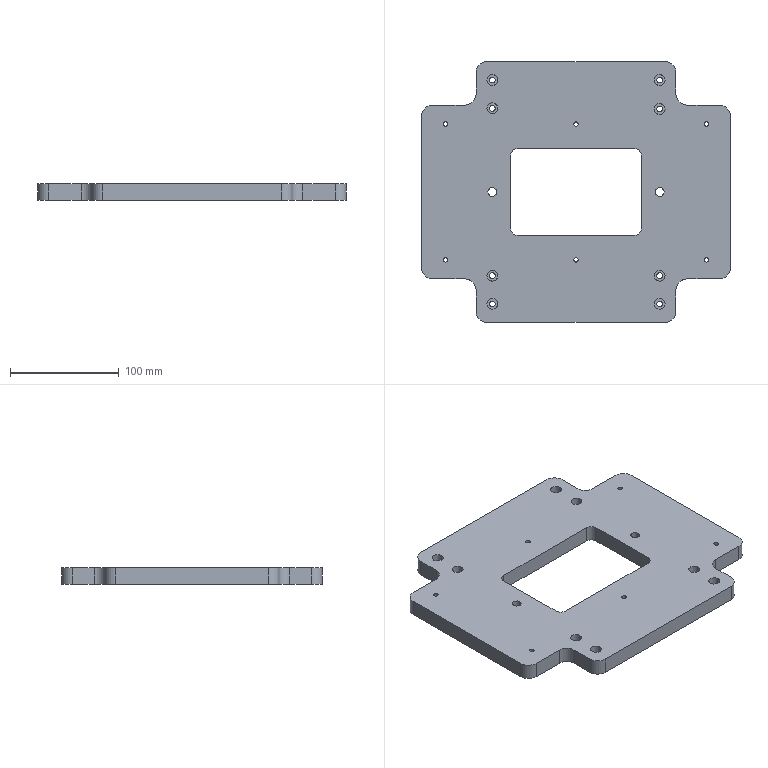NC program | NX | posted with a generic post | part box 284 x 240 x 15 mm
Lines 1 to 2692 of 2949, first 2174 of 2672 lines:
N10 G17 G21 G94 G90
(DRILLING , TOOL : D6A45)
N12 T07 M6
N14 G54
N16 G17 G0 G90 X0. Y-62.5 S5000 M3
N18 G43 Z30. H7
N20 G94 G81 G98 Z-1. F250. R3.
N22 X-77. Y-103.
N24 Y-77.
N26 X-120. Y-62.5
N28 X-77. Y0.
N30 X-120. Y62.5
N32 X-77. Y77.
N34 Y103.
N36 X0. Y62.5
N38 X77. Y103.
N40 Y76.337
N42 X120. Y62.5
N44 X77. Y0.
N46 X120. Y-62.5
N48 X77. Y-77.
N50 Y-103.
N52 G80
N54 G0 X77. Y-103. Z30.
N56 M5
(DRILLING_COPY , TOOL : 4.2ZT)
N58 T12 M6
N60 G54
N62 G17 G0 G90 X-120. Y62.5 S2000 M3
N64 G43 Z30. H12
N66 G94 G83 G98 Z-17.202 F200. Q2. R3.
N68 X0.
N70 X120.
N72 Y-62.5
N74 X0.
N76 X-120.
N78 G80
N80 G0 X-120. Y-62.5 Z30.
N82 M5
(DRILLING_COPY_1 , TOOL : 5.3ZT)
N84 T13 M6
N86 G54
N88 G17 G0 G90 X-77. Y-77. S2000 M3
N90 G43 Z30. H13
N92 G94 G83 G98 Z-17.592 F200. Q2. R3.
N94 Y-103.
N96 X77.
N98 Y-77.
N100 Y76.337
N102 Y103.
N104 X-77.
N106 Y77.
N108 G80
N110 G0 X-77. Y77. Z30.
N112 M5
(DRILLING_COPY_COPY , TOOL : 7.8ZT)
N114 T14 M6
N116 G54
N118 G17 G0 G90 X-77. Y0. S2000 M3
N120 G43 Z30. H14
N122 G94 G83 G98 Z-18.343 F200. Q2. R3.
N124 X77.
N126 G80
N128 G0 X77. Y0. Z30.
N130 M5
(HOLE_MILLING_1 , TOOL : D6)
N132 T06 M6
N134 G54
N136 G17 G0 G90 X-77. Y103. S9500 M3
N138 G43 Z30. H6
N140 Z0.5
N142 G94 G3 X-76. Y102. R1. F1600.
N144 X-75. Y103. R1.
N146 X-75. Y103. Z0. I-2. J0.
N148 X-75. Y103. Z-0.5 I-2. J0.
N150 X-75. Y103. Z-1. I-2. J0.
N152 X-75. Y103. Z-1.5 I-2. J0.
N154 X-75. Y103. Z-2. I-2. J0.
N156 X-75. Y103. Z-2.5 I-2. J0.
N158 X-75. Y103. Z-3. I-2. J0.
N160 X-75. Y103. Z-3.5 I-2. J0.
N162 X-75. Y103. Z-4. I-2. J0.
N164 X-75. Y103. Z-4.5 I-2. J0.
N166 X-75. Y103. Z-5. I-2. J0.
N168 X-75. Y103. Z-5.5 I-2. J0.
N170 X-75. Y103. Z-6. I-2. J0.
N172 X-75. Y103. Z-6.5 I-2. J0.
N174 X-75. Y103. Z-7. I-2. J0.
N176 X-75. Y103. Z-7.5 I-2. J0.
N178 X-75. Y103. Z-8. I-2. J0.
N180 X-75. Y103. Z-8.5 I-2. J0.
N182 X-75. Y103. Z-9. I-2. J0.
N184 X-75. Y103. Z-9.5 I-2. J0.
N186 X-75. Y103. Z-10. I-2. J0.
N188 X-75. Y103. Z-10.5 I-2. J0.
N190 X-75. Y103. Z-11. I-2. J0.
N192 X-75. Y103. Z-11.5 I-2. J0.
N194 X-75. Y103. Z-12. I-2. J0.
N196 X-77. Y105. R2.
N198 X-75. Y103. R-2.
N200 X-76. Y104. R1.
N202 X-77. Y103. R1.
N204 G0 Z30.
N206 Y77.
N208 Z0.5
N210 G3 X-76. Y76. R1.
N212 X-75. Y77. R1.
N214 X-75. Y77. Z0. I-2. J0.
N216 X-75. Y77. Z-0.5 I-2. J0.
N218 X-75. Y77. Z-1. I-2. J0.
N220 X-75. Y77. Z-1.5 I-2. J0.
N222 X-75. Y77. Z-2. I-2. J0.
N224 X-75. Y77. Z-2.5 I-2. J0.
N226 X-75. Y77. Z-3. I-2. J0.
N228 X-75. Y77. Z-3.5 I-2. J0.
N230 X-75. Y77. Z-4. I-2. J0.
N232 X-75. Y77. Z-4.5 I-2. J0.
N234 X-75. Y77. Z-5. I-2. J0.
N236 X-75. Y77. Z-5.5 I-2. J0.
N238 X-75. Y77. Z-6. I-2. J0.
N240 X-75. Y77. Z-6.5 I-2. J0.
N242 X-75. Y77. Z-7. I-2. J0.
N244 X-75. Y77. Z-7.5 I-2. J0.
N246 X-75. Y77. Z-8. I-2. J0.
N248 X-75. Y77. Z-8.5 I-2. J0.
N250 X-75. Y77. Z-9. I-2. J0.
N252 X-75. Y77. Z-9.5 I-2. J0.
N254 X-75. Y77. Z-10. I-2. J0.
N256 X-75. Y77. Z-10.5 I-2. J0.
N258 X-75. Y77. Z-11. I-2. J0.
N260 X-75. Y77. Z-11.5 I-2. J0.
N262 X-75. Y77. Z-12. I-2. J0.
N264 X-77. Y79. R2.
N266 X-75. Y77. R-2.
N268 X-76. Y78. R1.
N270 X-77. Y77. R1.
N272 G0 Z30.
N274 Y-77.
N276 Z0.5
N278 G3 X-76. Y-78. R1.
N280 X-75. Y-77. R1.
N282 X-75. Y-77. Z0. I-2. J0.
N284 X-75. Y-77. Z-0.5 I-2. J0.
N286 X-75. Y-77. Z-1. I-2. J0.
N288 X-75. Y-77. Z-1.5 I-2. J0.
N290 X-75. Y-77. Z-2. I-2. J0.
N292 X-75. Y-77. Z-2.5 I-2. J0.
N294 X-75. Y-77. Z-3. I-2. J0.
N296 X-75. Y-77. Z-3.5 I-2. J0.
N298 X-75. Y-77. Z-4. I-2. J0.
N300 X-75. Y-77. Z-4.5 I-2. J0.
N302 X-75. Y-77. Z-5. I-2. J0.
N304 X-75. Y-77. Z-5.5 I-2. J0.
N306 X-75. Y-77. Z-6. I-2. J0.
N308 X-75. Y-77. Z-6.5 I-2. J0.
N310 X-75. Y-77. Z-7. I-2. J0.
N312 X-75. Y-77. Z-7.5 I-2. J0.
N314 X-75. Y-77. Z-8. I-2. J0.
N316 X-75. Y-77. Z-8.5 I-2. J0.
N318 X-75. Y-77. Z-9. I-2. J0.
N320 X-75. Y-77. Z-9.5 I-2. J0.
N322 X-75. Y-77. Z-10. I-2. J0.
N324 X-75. Y-77. Z-10.5 I-2. J0.
N326 X-75. Y-77. Z-11. I-2. J0.
N328 X-75. Y-77. Z-11.5 I-2. J0.
N330 X-75. Y-77. Z-12. I-2. J0.
N332 X-77. Y-75. R2.
N334 X-75. Y-77. R-2.
N336 X-76. Y-76. R1.
N338 X-77. Y-77. R1.
N340 G0 Z30.
N342 Y-103.
N344 Z0.5
N346 G3 X-76. Y-104. R1.
N348 X-75. Y-103. R1.
N350 X-75. Y-103. Z0. I-2. J0.
N352 X-75. Y-103. Z-0.5 I-2. J0.
N354 X-75. Y-103. Z-1. I-2. J0.
N356 X-75. Y-103. Z-1.5 I-2. J0.
N358 X-75. Y-103. Z-2. I-2. J0.
N360 X-75. Y-103. Z-2.5 I-2. J0.
N362 X-75. Y-103. Z-3. I-2. J0.
N364 X-75. Y-103. Z-3.5 I-2. J0.
N366 X-75. Y-103. Z-4. I-2. J0.
N368 X-75. Y-103. Z-4.5 I-2. J0.
N370 X-75. Y-103. Z-5. I-2. J0.
N372 X-75. Y-103. Z-5.5 I-2. J0.
N374 X-75. Y-103. Z-6. I-2. J0.
N376 X-75. Y-103. Z-6.5 I-2. J0.
N378 X-75. Y-103. Z-7. I-2. J0.
N380 X-75. Y-103. Z-7.5 I-2. J0.
N382 X-75. Y-103. Z-8. I-2. J0.
N384 X-75. Y-103. Z-8.5 I-2. J0.
N386 X-75. Y-103. Z-9. I-2. J0.
N388 X-75. Y-103. Z-9.5 I-2. J0.
N390 X-75. Y-103. Z-10. I-2. J0.
N392 X-75. Y-103. Z-10.5 I-2. J0.
N394 X-75. Y-103. Z-11. I-2. J0.
N396 X-75. Y-103. Z-11.5 I-2. J0.
N398 X-75. Y-103. Z-12. I-2. J0.
N400 X-77. Y-101. R2.
N402 X-75. Y-103. R-2.
N404 X-76. Y-102. R1.
N406 X-77. Y-103. R1.
N408 G0 Z30.
N410 X77.
N412 Z0.5
N414 G3 X78. Y-104. R1.
N416 X79. Y-103. R1.
N418 X79. Y-103. Z0. I-2. J0.
N420 X79. Y-103. Z-0.5 I-2. J0.
N422 X79. Y-103. Z-1. I-2. J0.
N424 X79. Y-103. Z-1.5 I-2. J0.
N426 X79. Y-103. Z-2. I-2. J0.
N428 X79. Y-103. Z-2.5 I-2. J0.
N430 X79. Y-103. Z-3. I-2. J0.
N432 X79. Y-103. Z-3.5 I-2. J0.
N434 X79. Y-103. Z-4. I-2. J0.
N436 X79. Y-103. Z-4.5 I-2. J0.
N438 X79. Y-103. Z-5. I-2. J0.
N440 X79. Y-103. Z-5.5 I-2. J0.
N442 X79. Y-103. Z-6. I-2. J0.
N444 X79. Y-103. Z-6.5 I-2. J0.
N446 X79. Y-103. Z-7. I-2. J0.
N448 X79. Y-103. Z-7.5 I-2. J0.
N450 X79. Y-103. Z-8. I-2. J0.
N452 X79. Y-103. Z-8.5 I-2. J0.
N454 X79. Y-103. Z-9. I-2. J0.
N456 X79. Y-103. Z-9.5 I-2. J0.
N458 X79. Y-103. Z-10. I-2. J0.
N460 X79. Y-103. Z-10.5 I-2. J0.
N462 X79. Y-103. Z-11. I-2. J0.
N464 X79. Y-103. Z-11.5 I-2. J0.
N466 X79. Y-103. Z-12. I-2. J0.
N468 X77. Y-101. R2.
N470 X79. Y-103. R-2.
N472 X78. Y-102. R1.
N474 X77. Y-103. R1.
N476 G0 Z30.
N478 Y-77.
N480 Z0.5
N482 G3 X78. Y-78. R1.
N484 X79. Y-77. R1.
N486 X79. Y-77. Z0. I-2. J0.
N488 X79. Y-77. Z-0.5 I-2. J0.
N490 X79. Y-77. Z-1. I-2. J0.
N492 X79. Y-77. Z-1.5 I-2. J0.
N494 X79. Y-77. Z-2. I-2. J0.
N496 X79. Y-77. Z-2.5 I-2. J0.
N498 X79. Y-77. Z-3. I-2. J0.
N500 X79. Y-77. Z-3.5 I-2. J0.
N502 X79. Y-77. Z-4. I-2. J0.
N504 X79. Y-77. Z-4.5 I-2. J0.
N506 X79. Y-77. Z-5. I-2. J0.
N508 X79. Y-77. Z-5.5 I-2. J0.
N510 X79. Y-77. Z-6. I-2. J0.
N512 X79. Y-77. Z-6.5 I-2. J0.
N514 X79. Y-77. Z-7. I-2. J0.
N516 X79. Y-77. Z-7.5 I-2. J0.
N518 X79. Y-77. Z-8. I-2. J0.
N520 X79. Y-77. Z-8.5 I-2. J0.
N522 X79. Y-77. Z-9. I-2. J0.
N524 X79. Y-77. Z-9.5 I-2. J0.
N526 X79. Y-77. Z-10. I-2. J0.
N528 X79. Y-77. Z-10.5 I-2. J0.
N530 X79. Y-77. Z-11. I-2. J0.
N532 X79. Y-77. Z-11.5 I-2. J0.
N534 X79. Y-77. Z-12. I-2. J0.
N536 X77. Y-75. R2.
N538 X79. Y-77. R-2.
N540 X78. Y-76. R1.
N542 X77. Y-77. R1.
N544 G0 Z30.
N546 Y76.337
N548 Z0.5
N550 G3 X78. Y75.337 R1.
N552 X79. Y76.337 R1.
N554 X79. Y76.337 Z0. I-2. J0.
N556 X79. Y76.337 Z-0.5 I-2. J0.
N558 X79. Y76.337 Z-1. I-2. J0.
N560 X79. Y76.337 Z-1.5 I-2. J0.
N562 X79. Y76.337 Z-2. I-2. J0.
N564 X79. Y76.337 Z-2.5 I-2. J0.
N566 X79. Y76.337 Z-3. I-2. J0.
N568 X79. Y76.337 Z-3.5 I-2. J0.
N570 X79. Y76.337 Z-4. I-2. J0.
N572 X79. Y76.337 Z-4.5 I-2. J0.
N574 X79. Y76.337 Z-5. I-2. J0.
N576 X79. Y76.337 Z-5.5 I-2. J0.
N578 X79. Y76.337 Z-6. I-2. J0.
N580 X79. Y76.337 Z-6.5 I-2. J0.
N582 X79. Y76.337 Z-7. I-2. J0.
N584 X79. Y76.337 Z-7.5 I-2. J0.
N586 X79. Y76.337 Z-8. I-2. J0.
N588 X79. Y76.337 Z-8.5 I-2. J0.
N590 X79. Y76.337 Z-9. I-2. J0.
N592 X79. Y76.337 Z-9.5 I-2. J0.
N594 X79. Y76.337 Z-10. I-2. J0.
N596 X79. Y76.337 Z-10.5 I-2. J0.
N598 X79. Y76.337 Z-11. I-2. J0.
N600 X79. Y76.337 Z-11.5 I-2. J0.
N602 X79. Y76.337 Z-12. I-2. J0.
N604 X77. Y78.337 R2.
N606 X79. Y76.337 R-2.
N608 X78. Y77.337 R1.
N610 X77. Y76.337 R1.
N612 G0 Z30.
N614 Y103.
N616 Z0.5
N618 G3 X78. Y102. R1.
N620 X79. Y103. R1.
N622 X79. Y103. Z0. I-2. J0.
N624 X79. Y103. Z-0.5 I-2. J0.
N626 X79. Y103. Z-1. I-2. J0.
N628 X79. Y103. Z-1.5 I-2. J0.
N630 X79. Y103. Z-2. I-2. J0.
N632 X79. Y103. Z-2.5 I-2. J0.
N634 X79. Y103. Z-3. I-2. J0.
N636 X79. Y103. Z-3.5 I-2. J0.
N638 X79. Y103. Z-4. I-2. J0.
N640 X79. Y103. Z-4.5 I-2. J0.
N642 X79. Y103. Z-5. I-2. J0.
N644 X79. Y103. Z-5.5 I-2. J0.
N646 X79. Y103. Z-6. I-2. J0.
N648 X79. Y103. Z-6.5 I-2. J0.
N650 X79. Y103. Z-7. I-2. J0.
N652 X79. Y103. Z-7.5 I-2. J0.
N654 X79. Y103. Z-8. I-2. J0.
N656 X79. Y103. Z-8.5 I-2. J0.
N658 X79. Y103. Z-9. I-2. J0.
N660 X79. Y103. Z-9.5 I-2. J0.
N662 X79. Y103. Z-10. I-2. J0.
N664 X79. Y103. Z-10.5 I-2. J0.
N666 X79. Y103. Z-11. I-2. J0.
N668 X79. Y103. Z-11.5 I-2. J0.
N670 X79. Y103. Z-12. I-2. J0.
N672 X77. Y105. R2.
N674 X79. Y103. R-2.
N676 X78. Y104. R1.
N678 X77. Y103. R1.
N680 G0 Z30.
N682 M5
(PLANAR_MILL , TOOL : D10)
N684 T10 M6
N686 G54
N688 G17 G0 G90 X3.438 Y-0.4 S9500 M3
N690 G43 Z30. H10
N692 Z1.5
N694 G94 G1 X20.4 Z0.611 F1000.
N696 Y0.4 Z0.569
N698 X0. Z-0.5
N700 X-20.4 F3000.
N702 Y-0.4
N704 X20.4
N706 Y0.4
N708 X0.
N710 Y4.9
N712 X-24.9
N714 Y-4.9
N716 X24.9
N718 Y4.9
N720 X0.
N722 Y10.9
N724 X-30.9
N726 Y-10.9
N728 X30.9
N730 Y10.9
N732 X0.
N734 Y16.9
N736 X-36.9
N738 Y-16.9
N740 X36.9
N742 Y16.9
N744 X0.
N746 Y22.9
N748 X-42.9
N750 Y-22.9
N752 X42.9
N754 Y22.9
N756 X0.
N758 Y28.9
N760 X-48.9
N762 Y-28.9
N764 X48.9
N766 Y28.9
N768 X0.
N770 Y34.9
N772 X-54.
N774 G3 X-54.9 Y34. R0.9
N776 G1 Y-34.
N778 G3 X-54. Y-34.9 R0.9
N780 G1 X54.
N782 G3 X54.9 Y-34. R0.9
N784 G1 Y34.
N786 G3 X54. Y34.9 R0.9
N788 G1 X0.
N790 Z1.
N792 G0 X3.438 Y-0.4
N794 G1 X20.4 Z0.111 F1000.
N796 Y0.4 Z0.069
N798 X0. Z-1.
N800 X-20.4 F3000.
N802 Y-0.4
N804 X20.4
N806 Y0.4
N808 X0.
N810 Y4.9
N812 X-24.9
N814 Y-4.9
N816 X24.9
N818 Y4.9
N820 X0.
N822 Y10.9
N824 X-30.9
N826 Y-10.9
N828 X30.9
N830 Y10.9
N832 X0.
N834 Y16.9
N836 X-36.9
N838 Y-16.9
N840 X36.9
N842 Y16.9
N844 X0.
N846 Y22.9
N848 X-42.9
N850 Y-22.9
N852 X42.9
N854 Y22.9
N856 X0.
N858 Y28.9
N860 X-48.9
N862 Y-28.9
N864 X48.9
N866 Y28.9
N868 X0.
N870 Y34.9
N872 X-54.
N874 G3 X-54.9 Y34. R0.9
N876 G1 Y-34.
N878 G3 X-54. Y-34.9 R0.9
N880 G1 X54.
N882 G3 X54.9 Y-34. R0.9
N884 G1 Y34.
N886 G3 X54. Y34.9 R0.9
N888 G1 X0.
N890 Z0.5
N892 G0 X3.438 Y-0.4
N894 G1 X20.4 Z-0.389 F1000.
N896 Y0.4 Z-0.431
N898 X0. Z-1.5
N900 X-20.4 F3000.
N902 Y-0.4
N904 X20.4
N906 Y0.4
N908 X0.
N910 Y4.9
N912 X-24.9
N914 Y-4.9
N916 X24.9
N918 Y4.9
N920 X0.
N922 Y10.9
N924 X-30.9
N926 Y-10.9
N928 X30.9
N930 Y10.9
N932 X0.
N934 Y16.9
N936 X-36.9
N938 Y-16.9
N940 X36.9
N942 Y16.9
N944 X0.
N946 Y22.9
N948 X-42.9
N950 Y-22.9
N952 X42.9
N954 Y22.9
N956 X0.
N958 Y28.9
N960 X-48.9
N962 Y-28.9
N964 X48.9
N966 Y28.9
N968 X0.
N970 Y34.9
N972 X-54.
N974 G3 X-54.9 Y34. R0.9
N976 G1 Y-34.
N978 G3 X-54. Y-34.9 R0.9
N980 G1 X54.
N982 G3 X54.9 Y-34. R0.9
N984 G1 Y34.
N986 G3 X54. Y34.9 R0.9
N988 G1 X0.
N990 Z0.
N992 G0 X3.438 Y-0.4
N994 G1 X20.4 Z-0.889 F1000.
N996 Y0.4 Z-0.931
N998 X0. Z-2.
N1000 X-20.4 F3000.
N1002 Y-0.4
N1004 X20.4
N1006 Y0.4
N1008 X0.
N1010 Y4.9
N1012 X-24.9
N1014 Y-4.9
N1016 X24.9
N1018 Y4.9
N1020 X0.
N1022 Y10.9
N1024 X-30.9
N1026 Y-10.9
N1028 X30.9
N1030 Y10.9
N1032 X0.
N1034 Y16.9
N1036 X-36.9
N1038 Y-16.9
N1040 X36.9
N1042 Y16.9
N1044 X0.
N1046 Y22.9
N1048 X-42.9
N1050 Y-22.9
N1052 X42.9
N1054 Y22.9
N1056 X0.
N1058 Y28.9
N1060 X-48.9
N1062 Y-28.9
N1064 X48.9
N1066 Y28.9
N1068 X0.
N1070 Y34.9
N1072 X-54.
N1074 G3 X-54.9 Y34. R0.9
N1076 G1 Y-34.
N1078 G3 X-54. Y-34.9 R0.9
N1080 G1 X54.
N1082 G3 X54.9 Y-34. R0.9
N1084 G1 Y34.
N1086 G3 X54. Y34.9 R0.9
N1088 G1 X0.
N1090 Z-0.5
N1092 G0 X3.438 Y-0.4
N1094 G1 X20.4 Z-1.389 F1000.
N1096 Y0.4 Z-1.431
N1098 X0. Z-2.5
N1100 X-20.4 F3000.
N1102 Y-0.4
N1104 X20.4
N1106 Y0.4
N1108 X0.
N1110 Y4.9
N1112 X-24.9
N1114 Y-4.9
N1116 X24.9
N1118 Y4.9
N1120 X0.
N1122 Y10.9
N1124 X-30.9
N1126 Y-10.9
N1128 X30.9
N1130 Y10.9
N1132 X0.
N1134 Y16.9
N1136 X-36.9
N1138 Y-16.9
N1140 X36.9
N1142 Y16.9
N1144 X0.
N1146 Y22.9
N1148 X-42.9
N1150 Y-22.9
N1152 X42.9
N1154 Y22.9
N1156 X0.
N1158 Y28.9
N1160 X-48.9
N1162 Y-28.9
N1164 X48.9
N1166 Y28.9
N1168 X0.
N1170 Y34.9
N1172 X-54.
N1174 G3 X-54.9 Y34. R0.9
N1176 G1 Y-34.
N1178 G3 X-54. Y-34.9 R0.9
N1180 G1 X54.
N1182 G3 X54.9 Y-34. R0.9
N1184 G1 Y34.
N1186 G3 X54. Y34.9 R0.9
N1188 G1 X0.
N1190 Z-1.
N1192 G0 X3.438 Y-0.4
N1194 G1 X20.4 Z-1.889 F1000.
N1196 Y0.4 Z-1.931
N1198 X0. Z-3.
N1200 X-20.4 F3000.
N1202 Y-0.4
N1204 X20.4
N1206 Y0.4
N1208 X0.
N1210 Y4.9
N1212 X-24.9
N1214 Y-4.9
N1216 X24.9
N1218 Y4.9
N1220 X0.
N1222 Y10.9
N1224 X-30.9
N1226 Y-10.9
N1228 X30.9
N1230 Y10.9
N1232 X0.
N1234 Y16.9
N1236 X-36.9
N1238 Y-16.9
N1240 X36.9
N1242 Y16.9
N1244 X0.
N1246 Y22.9
N1248 X-42.9
N1250 Y-22.9
N1252 X42.9
N1254 Y22.9
N1256 X0.
N1258 Y28.9
N1260 X-48.9
N1262 Y-28.9
N1264 X48.9
N1266 Y28.9
N1268 X0.
N1270 Y34.9
N1272 X-54.
N1274 G3 X-54.9 Y34. R0.9
N1276 G1 Y-34.
N1278 G3 X-54. Y-34.9 R0.9
N1280 G1 X54.
N1282 G3 X54.9 Y-34. R0.9
N1284 G1 Y34.
N1286 G3 X54. Y34.9 R0.9
N1288 G1 X0.
N1290 Z-1.5
N1292 G0 X3.438 Y-0.4
N1294 G1 X20.4 Z-2.389 F1000.
N1296 Y0.4 Z-2.431
N1298 X0. Z-3.5
N1300 X-20.4 F3000.
N1302 Y-0.4
N1304 X20.4
N1306 Y0.4
N1308 X0.
N1310 Y4.9
N1312 X-24.9
N1314 Y-4.9
N1316 X24.9
N1318 Y4.9
N1320 X0.
N1322 Y10.9
N1324 X-30.9
N1326 Y-10.9
N1328 X30.9
N1330 Y10.9
N1332 X0.
N1334 Y16.9
N1336 X-36.9
N1338 Y-16.9
N1340 X36.9
N1342 Y16.9
N1344 X0.
N1346 Y22.9
N1348 X-42.9
N1350 Y-22.9
N1352 X42.9
N1354 Y22.9
N1356 X0.
N1358 Y28.9
N1360 X-48.9
N1362 Y-28.9
N1364 X48.9
N1366 Y28.9
N1368 X0.
N1370 Y34.9
N1372 X-54.
N1374 G3 X-54.9 Y34. R0.9
N1376 G1 Y-34.
N1378 G3 X-54. Y-34.9 R0.9
N1380 G1 X54.
N1382 G3 X54.9 Y-34. R0.9
N1384 G1 Y34.
N1386 G3 X54. Y34.9 R0.9
N1388 G1 X0.
N1390 Z-2.
N1392 G0 X3.438 Y-0.4
N1394 G1 X20.4 Z-2.889 F1000.
N1396 Y0.4 Z-2.931
N1398 X0. Z-4.
N1400 X-20.4 F3000.
N1402 Y-0.4
N1404 X20.4
N1406 Y0.4
N1408 X0.
N1410 Y4.9
N1412 X-24.9
N1414 Y-4.9
N1416 X24.9
N1418 Y4.9
N1420 X0.
N1422 Y10.9
N1424 X-30.9
N1426 Y-10.9
N1428 X30.9
N1430 Y10.9
N1432 X0.
N1434 Y16.9
N1436 X-36.9
N1438 Y-16.9
N1440 X36.9
N1442 Y16.9
N1444 X0.
N1446 Y22.9
N1448 X-42.9
N1450 Y-22.9
N1452 X42.9
N1454 Y22.9
N1456 X0.
N1458 Y28.9
N1460 X-48.9
N1462 Y-28.9
N1464 X48.9
N1466 Y28.9
N1468 X0.
N1470 Y34.9
N1472 X-54.
N1474 G3 X-54.9 Y34. R0.9
N1476 G1 Y-34.
N1478 G3 X-54. Y-34.9 R0.9
N1480 G1 X54.
N1482 G3 X54.9 Y-34. R0.9
N1484 G1 Y34.
N1486 G3 X54. Y34.9 R0.9
N1488 G1 X0.
N1490 Z-2.5
N1492 G0 X3.438 Y-0.4
N1494 G1 X20.4 Z-3.389 F1000.
N1496 Y0.4 Z-3.431
N1498 X0. Z-4.5
N1500 X-20.4 F3000.
N1502 Y-0.4
N1504 X20.4
N1506 Y0.4
N1508 X0.
N1510 Y4.9
N1512 X-24.9
N1514 Y-4.9
N1516 X24.9
N1518 Y4.9
N1520 X0.
N1522 Y10.9
N1524 X-30.9
N1526 Y-10.9
N1528 X30.9
N1530 Y10.9
N1532 X0.
N1534 Y16.9
N1536 X-36.9
N1538 Y-16.9
N1540 X36.9
N1542 Y16.9
N1544 X0.
N1546 Y22.9
N1548 X-42.9
N1550 Y-22.9
N1552 X42.9
N1554 Y22.9
N1556 X0.
N1558 Y28.9
N1560 X-48.9
N1562 Y-28.9
N1564 X48.9
N1566 Y28.9
N1568 X0.
N1570 Y34.9
N1572 X-54.
N1574 G3 X-54.9 Y34. R0.9
N1576 G1 Y-34.
N1578 G3 X-54. Y-34.9 R0.9
N1580 G1 X54.
N1582 G3 X54.9 Y-34. R0.9
N1584 G1 Y34.
N1586 G3 X54. Y34.9 R0.9
N1588 G1 X0.
N1590 Z-3.
N1592 G0 X3.438 Y-0.4
N1594 G1 X20.4 Z-3.889 F1000.
N1596 Y0.4 Z-3.931
N1598 X0. Z-5.
N1600 X-20.4 F3000.
N1602 Y-0.4
N1604 X20.4
N1606 Y0.4
N1608 X0.
N1610 Y4.9
N1612 X-24.9
N1614 Y-4.9
N1616 X24.9
N1618 Y4.9
N1620 X0.
N1622 Y10.9
N1624 X-30.9
N1626 Y-10.9
N1628 X30.9
N1630 Y10.9
N1632 X0.
N1634 Y16.9
N1636 X-36.9
N1638 Y-16.9
N1640 X36.9
N1642 Y16.9
N1644 X0.
N1646 Y22.9
N1648 X-42.9
N1650 Y-22.9
N1652 X42.9
N1654 Y22.9
N1656 X0.
N1658 Y28.9
N1660 X-48.9
N1662 Y-28.9
N1664 X48.9
N1666 Y28.9
N1668 X0.
N1670 Y34.9
N1672 X-54.
N1674 G3 X-54.9 Y34. R0.9
N1676 G1 Y-34.
N1678 G3 X-54. Y-34.9 R0.9
N1680 G1 X54.
N1682 G3 X54.9 Y-34. R0.9
N1684 G1 Y34.
N1686 G3 X54. Y34.9 R0.9
N1688 G1 X0.
N1690 Z-3.5
N1692 G0 X3.438 Y-0.4
N1694 G1 X20.4 Z-4.389 F1000.
N1696 Y0.4 Z-4.431
N1698 X0. Z-5.5
N1700 X-20.4 F3000.
N1702 Y-0.4
N1704 X20.4
N1706 Y0.4
N1708 X0.
N1710 Y4.9
N1712 X-24.9
N1714 Y-4.9
N1716 X24.9
N1718 Y4.9
N1720 X0.
N1722 Y10.9
N1724 X-30.9
N1726 Y-10.9
N1728 X30.9
N1730 Y10.9
N1732 X0.
N1734 Y16.9
N1736 X-36.9
N1738 Y-16.9
N1740 X36.9
N1742 Y16.9
N1744 X0.
N1746 Y22.9
N1748 X-42.9
N1750 Y-22.9
N1752 X42.9
N1754 Y22.9
N1756 X0.
N1758 Y28.9
N1760 X-48.9
N1762 Y-28.9
N1764 X48.9
N1766 Y28.9
N1768 X0.
N1770 Y34.9
N1772 X-54.
N1774 G3 X-54.9 Y34. R0.9
N1776 G1 Y-34.
N1778 G3 X-54. Y-34.9 R0.9
N1780 G1 X54.
N1782 G3 X54.9 Y-34. R0.9
N1784 G1 Y34.
N1786 G3 X54. Y34.9 R0.9
N1788 G1 X0.
N1790 Z-4.
N1792 G0 X3.438 Y-0.4
N1794 G1 X20.4 Z-4.889 F1000.
N1796 Y0.4 Z-4.931
N1798 X0. Z-6.
N1800 X-20.4 F3000.
N1802 Y-0.4
N1804 X20.4
N1806 Y0.4
N1808 X0.
N1810 Y4.9
N1812 X-24.9
N1814 Y-4.9
N1816 X24.9
N1818 Y4.9
N1820 X0.
N1822 Y10.9
N1824 X-30.9
N1826 Y-10.9
N1828 X30.9
N1830 Y10.9
N1832 X0.
N1834 Y16.9
N1836 X-36.9
N1838 Y-16.9
N1840 X36.9
N1842 Y16.9
N1844 X0.
N1846 Y22.9
N1848 X-42.9
N1850 Y-22.9
N1852 X42.9
N1854 Y22.9
N1856 X0.
N1858 Y28.9
N1860 X-48.9
N1862 Y-28.9
N1864 X48.9
N1866 Y28.9
N1868 X0.
N1870 Y34.9
N1872 X-54.
N1874 G3 X-54.9 Y34. R0.9
N1876 G1 Y-34.
N1878 G3 X-54. Y-34.9 R0.9
N1880 G1 X54.
N1882 G3 X54.9 Y-34. R0.9
N1884 G1 Y34.
N1886 G3 X54. Y34.9 R0.9
N1888 G1 X0.
N1890 Z-4.5
N1892 G0 X3.438 Y-0.4
N1894 G1 X20.4 Z-5.389 F1000.
N1896 Y0.4 Z-5.431
N1898 X0. Z-6.5
N1900 X-20.4 F3000.
N1902 Y-0.4
N1904 X20.4
N1906 Y0.4
N1908 X0.
N1910 Y4.9
N1912 X-24.9
N1914 Y-4.9
N1916 X24.9
N1918 Y4.9
N1920 X0.
N1922 Y10.9
N1924 X-30.9
N1926 Y-10.9
N1928 X30.9
N1930 Y10.9
N1932 X0.
N1934 Y16.9
N1936 X-36.9
N1938 Y-16.9
N1940 X36.9
N1942 Y16.9
N1944 X0.
N1946 Y22.9
N1948 X-42.9
N1950 Y-22.9
N1952 X42.9
N1954 Y22.9
N1956 X0.
N1958 Y28.9
N1960 X-48.9
N1962 Y-28.9
N1964 X48.9
N1966 Y28.9
N1968 X0.
N1970 Y34.9
N1972 X-54.
N1974 G3 X-54.9 Y34. R0.9
N1976 G1 Y-34.
N1978 G3 X-54. Y-34.9 R0.9
N1980 G1 X54.
N1982 G3 X54.9 Y-34. R0.9
N1984 G1 Y34.
N1986 G3 X54. Y34.9 R0.9
N1988 G1 X0.
N1990 Z-5.
N1992 G0 X3.438 Y-0.4
N1994 G1 X20.4 Z-5.889 F1000.
N1996 Y0.4 Z-5.931
N1998 X0. Z-7.
N2000 X-20.4 F3000.
N2002 Y-0.4
N2004 X20.4
N2006 Y0.4
N2008 X0.
N2010 Y4.9
N2012 X-24.9
N2014 Y-4.9
N2016 X24.9
N2018 Y4.9
N2020 X0.
N2022 Y10.9
N2024 X-30.9
N2026 Y-10.9
N2028 X30.9
N2030 Y10.9
N2032 X0.
N2034 Y16.9
N2036 X-36.9
N2038 Y-16.9
N2040 X36.9
N2042 Y16.9
N2044 X0.
N2046 Y22.9
N2048 X-42.9
N2050 Y-22.9
N2052 X42.9
N2054 Y22.9
N2056 X0.
N2058 Y28.9
N2060 X-48.9
N2062 Y-28.9
N2064 X48.9
N2066 Y28.9
N2068 X0.
N2070 Y34.9
N2072 X-54.
N2074 G3 X-54.9 Y34. R0.9
N2076 G1 Y-34.
N2078 G3 X-54. Y-34.9 R0.9
N2080 G1 X54.
N2082 G3 X54.9 Y-34. R0.9
N2084 G1 Y34.
N2086 G3 X54. Y34.9 R0.9
N2088 G1 X0.
N2090 Z-5.5
N2092 G0 X3.438 Y-0.4
N2094 G1 X20.4 Z-6.389 F1000.
N2096 Y0.4 Z-6.431
N2098 X0. Z-7.5
N2100 X-20.4 F3000.
N2102 Y-0.4
N2104 X20.4
N2106 Y0.4
N2108 X0.
N2110 Y4.9
N2112 X-24.9
N2114 Y-4.9
N2116 X24.9
N2118 Y4.9
N2120 X0.
N2122 Y10.9
N2124 X-30.9
N2126 Y-10.9
N2128 X30.9
N2130 Y10.9
N2132 X0.
N2134 Y16.9
N2136 X-36.9
N2138 Y-16.9
N2140 X36.9
N2142 Y16.9
N2144 X0.
N2146 Y22.9
N2148 X-42.9
N2150 Y-22.9
N2152 X42.9
N2154 Y22.9
N2156 X0.
N2158 Y28.9
N2160 X-48.9
N2162 Y-28.9
N2164 X48.9
N2166 Y28.9
N2168 X0.
N2170 Y34.9
N2172 X-54.
N2174 G3 X-54.9 Y34. R0.9
N2176 G1 Y-34.
N2178 G3 X-54. Y-34.9 R0.9
N2180 G1 X54.
N2182 G3 X54.9 Y-34. R0.9
N2184 G1 Y34.
N2186 G3 X54. Y34.9 R0.9
N2188 G1 X0.
N2190 Z-6.
N2192 G0 X3.438 Y-0.4
N2194 G1 X20.4 Z-6.889 F1000.
N2196 Y0.4 Z-6.931
N2198 X0. Z-8.
N2200 X-20.4 F3000.
N2202 Y-0.4
N2204 X20.4
N2206 Y0.4
N2208 X0.
N2210 Y4.9
N2212 X-24.9
N2214 Y-4.9
N2216 X24.9
N2218 Y4.9
N2220 X0.
N2222 Y10.9
N2224 X-30.9
N2226 Y-10.9
N2228 X30.9
N2230 Y10.9
N2232 X0.
N2234 Y16.9
N2236 X-36.9
N2238 Y-16.9
N2240 X36.9
N2242 Y16.9
N2244 X0.
N2246 Y22.9
N2248 X-42.9
N2250 Y-22.9
N2252 X42.9
N2254 Y22.9
N2256 X0.
N2258 Y28.9
N2260 X-48.9
N2262 Y-28.9
N2264 X48.9
N2266 Y28.9
N2268 X0.
N2270 Y34.9
N2272 X-54.
N2274 G3 X-54.9 Y34. R0.9
N2276 G1 Y-34.
N2278 G3 X-54. Y-34.9 R0.9
N2280 G1 X54.
N2282 G3 X54.9 Y-34. R0.9
N2284 G1 Y34.
N2286 G3 X54. Y34.9 R0.9
N2288 G1 X0.
N2290 Z-6.5
N2292 G0 X3.438 Y-0.4
N2294 G1 X20.4 Z-7.389 F1000.
N2296 Y0.4 Z-7.431
N2298 X0. Z-8.5
N2300 X-20.4 F3000.
N2302 Y-0.4
N2304 X20.4
N2306 Y0.4
N2308 X0.
N2310 Y4.9
N2312 X-24.9
N2314 Y-4.9
N2316 X24.9
N2318 Y4.9
N2320 X0.
N2322 Y10.9
N2324 X-30.9
N2326 Y-10.9
N2328 X30.9
N2330 Y10.9
N2332 X0.
N2334 Y16.9
N2336 X-36.9
N2338 Y-16.9
N2340 X36.9
N2342 Y16.9
N2344 X0.
N2346 Y22.9
N2348 X-42.9
N2350 Y-22.9
N2352 X42.9
N2354 Y22.9
N2356 X0.
N2358 Y28.9
N2360 X-48.9
N2362 Y-28.9
N2364 X48.9
N2366 Y28.9
N2368 X0.
N2370 Y34.9
N2372 X-54.
N2374 G3 X-54.9 Y34. R0.9
N2376 G1 Y-34.
N2378 G3 X-54. Y-34.9 R0.9
N2380 G1 X54.
N2382 G3 X54.9 Y-34. R0.9
N2384 G1 Y34.
N2386 G3 X54. Y34.9 R0.9
N2388 G1 X0.
N2390 Z-7.
N2392 G0 X3.438 Y-0.4
N2394 G1 X20.4 Z-7.889 F1000.
N2396 Y0.4 Z-7.931
N2398 X0. Z-9.
N2400 X-20.4 F3000.
N2402 Y-0.4
N2404 X20.4
N2406 Y0.4
N2408 X0.
N2410 Y4.9
N2412 X-24.9
N2414 Y-4.9
N2416 X24.9
N2418 Y4.9
N2420 X0.
N2422 Y10.9
N2424 X-30.9
N2426 Y-10.9
N2428 X30.9
N2430 Y10.9
N2432 X0.
N2434 Y16.9
N2436 X-36.9
N2438 Y-16.9
N2440 X36.9
N2442 Y16.9
N2444 X0.
N2446 Y22.9
N2448 X-42.9
N2450 Y-22.9
N2452 X42.9
N2454 Y22.9
N2456 X0.
N2458 Y28.9
N2460 X-48.9
N2462 Y-28.9
N2464 X48.9
N2466 Y28.9
N2468 X0.
N2470 Y34.9
N2472 X-54.
N2474 G3 X-54.9 Y34. R0.9
N2476 G1 Y-34.
N2478 G3 X-54. Y-34.9 R0.9
N2480 G1 X54.
N2482 G3 X54.9 Y-34. R0.9
N2484 G1 Y34.
N2486 G3 X54. Y34.9 R0.9
N2488 G1 X0.
N2490 Z-7.5
N2492 G0 X3.438 Y-0.4
N2494 G1 X20.4 Z-8.389 F1000.
N2496 Y0.4 Z-8.431
N2498 X0. Z-9.5
N2500 X-20.4 F3000.
N2502 Y-0.4
N2504 X20.4
N2506 Y0.4
N2508 X0.
N2510 Y4.9
N2512 X-24.9
N2514 Y-4.9
N2516 X24.9
N2518 Y4.9
N2520 X0.
N2522 Y10.9
N2524 X-30.9
N2526 Y-10.9
N2528 X30.9
N2530 Y10.9
N2532 X0.
N2534 Y16.9
N2536 X-36.9
N2538 Y-16.9
N2540 X36.9
N2542 Y16.9
N2544 X0.
N2546 Y22.9
N2548 X-42.9
N2550 Y-22.9
N2552 X42.9
N2554 Y22.9
N2556 X0.
N2558 Y28.9
N2560 X-48.9
N2562 Y-28.9
N2564 X48.9
N2566 Y28.9
N2568 X0.
N2570 Y34.9
N2572 X-54.
N2574 G3 X-54.9 Y34. R0.9
N2576 G1 Y-34.
N2578 G3 X-54. Y-34.9 R0.9
N2580 G1 X54.
N2582 G3 X54.9 Y-34. R0.9
N2584 G1 Y34.
N2586 G3 X54. Y34.9 R0.9
N2588 G1 X0.
N2590 Z-8.
N2592 G0 X3.438 Y-0.4
N2594 G1 X20.4 Z-8.889 F1000.
N2596 Y0.4 Z-8.931
N2598 X0. Z-10.
N2600 X-20.4 F3000.
N2602 Y-0.4
N2604 X20.4
N2606 Y0.4
N2608 X0.
N2610 Y4.9
N2612 X-24.9
N2614 Y-4.9
N2616 X24.9
N2618 Y4.9
N2620 X0.
N2622 Y10.9
N2624 X-30.9
N2626 Y-10.9
N2628 X30.9
N2630 Y10.9
N2632 X0.
N2634 Y16.9
N2636 X-36.9
N2638 Y-16.9
N2640 X36.9
N2642 Y16.9
N2644 X0.
N2646 Y22.9
N2648 X-42.9
N2650 Y-22.9
N2652 X42.9
N2654 Y22.9
N2656 X0.
N2658 Y28.9
N2660 X-48.9
N2662 Y-28.9
N2664 X48.9
N2666 Y28.9
N2668 X0.
N2670 Y34.9
N2672 X-54.
N2674 G3 X-54.9 Y34. R0.9
N2676 G1 Y-34.
N2678 G3 X-54. Y-34.9 R0.9
N2680 G1 X54.
N2682 G3 X54.9 Y-34. R0.9
N2684 G1 Y34.
N2686 G3 X54. Y34.9 R0.9
N2688 G1 X0.
N2690 Z-8.5
N2692 G0 X3.438 Y-0.4
N2694 G1 X20.4 Z-9.389 F1000.
N2696 Y0.4 Z-9.431
N2698 X0. Z-10.5
N2700 X-20.4 F3000.
N2702 Y-0.4
N2704 X20.4
N2706 Y0.4
N2708 X0.
N2710 Y4.9
N2712 X-24.9
N2714 Y-4.9
N2716 X24.9
N2718 Y4.9
N2720 X0.
N2722 Y10.9
N2724 X-30.9
N2726 Y-10.9
N2728 X30.9
N2730 Y10.9
N2732 X0.
N2734 Y16.9
N2736 X-36.9
N2738 Y-16.9
N2740 X36.9
N2742 Y16.9
N2744 X0.
N2746 Y22.9
N2748 X-42.9
N2750 Y-22.9
N2752 X42.9
N2754 Y22.9
N2756 X0.
N2758 Y28.9
N2760 X-48.9
N2762 Y-28.9
N2764 X48.9
N2766 Y28.9
N2768 X0.
N2770 Y34.9
N2772 X-54.
N2774 G3 X-54.9 Y34. R0.9
N2776 G1 Y-34.
N2778 G3 X-54. Y-34.9 R0.9
N2780 G1 X54.
N2782 G3 X54.9 Y-34. R0.9
N2784 G1 Y34.
N2786 G3 X54. Y34.9 R0.9
N2788 G1 X0.
N2790 Z-9.
N2792 G0 X3.438 Y-0.4
N2794 G1 X20.4 Z-9.889 F1000.
N2796 Y0.4 Z-9.931
N2798 X0. Z-11.
N2800 X-20.4 F3000.
N2802 Y-0.4
N2804 X20.4
N2806 Y0.4
N2808 X0.
N2810 Y4.9
N2812 X-24.9
N2814 Y-4.9
N2816 X24.9
N2818 Y4.9
N2820 X0.
N2822 Y10.9
N2824 X-30.9
N2826 Y-10.9
N2828 X30.9
N2830 Y10.9
N2832 X0.
N2834 Y16.9
N2836 X-36.9
N2838 Y-16.9
N2840 X36.9
N2842 Y16.9
N2844 X0.
N2846 Y22.9
N2848 X-42.9
N2850 Y-22.9
N2852 X42.9
N2854 Y22.9
N2856 X0.
N2858 Y28.9
N2860 X-48.9
N2862 Y-28.9
N2864 X48.9
N2866 Y28.9
N2868 X0.
N2870 Y34.9
N2872 X-54.
N2874 G3 X-54.9 Y34. R0.9
N2876 G1 Y-34.
N2878 G3 X-54. Y-34.9 R0.9
N2880 G1 X54.
N2882 G3 X54.9 Y-34. R0.9
N2884 G1 Y34.
N2886 G3 X54. Y34.9 R0.9
N2888 G1 X0.
N2890 Z-9.5
N2892 G0 X3.438 Y-0.4
N2894 G1 X20.4 Z-10.389 F1000.
N2896 Y0.4 Z-10.431
N2898 X0. Z-11.5
N2900 X-20.4 F3000.
N2902 Y-0.4
N2904 X20.4
N2906 Y0.4
N2908 X0.
N2910 Y4.9
N2912 X-24.9
N2914 Y-4.9
N2916 X24.9
N2918 Y4.9
N2920 X0.
N2922 Y10.9
N2924 X-30.9
N2926 Y-10.9
N2928 X30.9
N2930 Y10.9
N2932 X0.
N2934 Y16.9
N2936 X-36.9
N2938 Y-16.9
N2940 X36.9
N2942 Y16.9
N2944 X0.
N2946 Y22.9
N2948 X-42.9
N2950 Y-22.9
N2952 X42.9
N2954 Y22.9
N2956 X0.
N2958 Y28.9
N2960 X-48.9
N2962 Y-28.9
N2964 X48.9
N2966 Y28.9
N2968 X0.
N2970 Y34.9
N2972 X-54.
N2974 G3 X-54.9 Y34. R0.9
N2976 G1 Y-34.
N2978 G3 X-54. Y-34.9 R0.9
N2980 G1 X54.
N2982 G3 X54.9 Y-34. R0.9
N2984 G1 Y34.
N2986 G3 X54. Y34.9 R0.9
N2988 G1 X0.
N2990 Z-10.
N2992 G0 X3.438 Y-0.4
N2994 G1 X20.4 Z-10.889 F1000.
N2996 Y0.4 Z-10.931
N2998 X0. Z-12.
N3000 X-20.4 F3000.
N3002 Y-0.4
N3004 X20.4
N3006 Y0.4
N3008 X0.
N3010 Y4.9
N3012 X-24.9
N3014 Y-4.9
N3016 X24.9
N3018 Y4.9
N3020 X0.
N3022 Y10.9
N3024 X-30.9
N3026 Y-10.9
N3028 X30.9
N3030 Y10.9
N3032 X0.
N3034 Y16.9
N3036 X-36.9
N3038 Y-16.9
N3040 X36.9
N3042 Y16.9
N3044 X0.
N3046 Y22.9
N3048 X-42.9
N3050 Y-22.9
N3052 X42.9
N3054 Y22.9
N3056 X0.
N3058 Y28.9
N3060 X-48.9
N3062 Y-28.9
N3064 X48.9
N3066 Y28.9
N3068 X0.
N3070 Y34.9
N3072 X-54.
N3074 G3 X-54.9 Y34. R0.9
N3076 G1 Y-34.
N3078 G3 X-54. Y-34.9 R0.9
N3080 G1 X54.
N3082 G3 X54.9 Y-34. R0.9
N3084 G1 Y34.
N3086 G3 X54. Y34.9 R0.9
N3088 G1 X0.
N3090 Z-10.5
N3092 G0 X3.438 Y-0.4
N3094 G1 X20.4 Z-11.389 F1000.
N3096 Y0.4 Z-11.431
N3098 X0. Z-12.5
N3100 X-20.4 F3000.
N3102 Y-0.4
N3104 X20.4
N3106 Y0.4
N3108 X0.
N3110 Y4.9
N3112 X-24.9
N3114 Y-4.9
N3116 X24.9
N3118 Y4.9
N3120 X0.
N3122 Y10.9
N3124 X-30.9
N3126 Y-10.9
N3128 X30.9
N3130 Y10.9
N3132 X0.
N3134 Y16.9
N3136 X-36.9
N3138 Y-16.9
N3140 X36.9
N3142 Y16.9
N3144 X0.
N3146 Y22.9
N3148 X-42.9
N3150 Y-22.9
N3152 X42.9
N3154 Y22.9
N3156 X0.
N3158 Y28.9
N3160 X-48.9
N3162 Y-28.9
N3164 X48.9
N3166 Y28.9
N3168 X0.
N3170 Y34.9
N3172 X-54.
N3174 G3 X-54.9 Y34. R0.9
N3176 G1 Y-34.
N3178 G3 X-54. Y-34.9 R0.9
N3180 G1 X54.
N3182 G3 X54.9 Y-34. R0.9
N3184 G1 Y34.
N3186 G3 X54. Y34.9 R0.9
N3188 G1 X0.
N3190 Z-11.
N3192 G0 X3.438 Y-0.4
N3194 G1 X20.4 Z-11.889 F1000.
N3196 Y0.4 Z-11.931
N3198 X0. Z-13.
N3200 X-20.4 F3000.
N3202 Y-0.4
N3204 X20.4
N3206 Y0.4
N3208 X0.
N3210 Y4.9
N3212 X-24.9
N3214 Y-4.9
N3216 X24.9
N3218 Y4.9
N3220 X0.
N3222 Y10.9
N3224 X-30.9
N3226 Y-10.9
N3228 X30.9
N3230 Y10.9
N3232 X0.
N3234 Y16.9
N3236 X-36.9
N3238 Y-16.9
N3240 X36.9
N3242 Y16.9
N3244 X0.
N3246 Y22.9
N3248 X-42.9
N3250 Y-22.9
N3252 X42.9
N3254 Y22.9
N3256 X0.
N3258 Y28.9
N3260 X-48.9
N3262 Y-28.9
N3264 X48.9
N3266 Y28.9
N3268 X0.
N3270 Y34.9
N3272 X-54.
N3274 G3 X-54.9 Y34. R0.9
N3276 G1 Y-34.
N3278 G3 X-54. Y-34.9 R0.9
N3280 G1 X54.
N3282 G3 X54.9 Y-34. R0.9
N3284 G1 Y34.
N3286 G3 X54. Y34.9 R0.9
N3288 G1 X0.
N3290 Z-11.5
N3292 G0 X3.438 Y-0.4
N3294 G1 X20.4 Z-12.389 F1000.
N3296 Y0.4 Z-12.431
N3298 X0. Z-13.5
N3300 X-20.4 F3000.
N3302 Y-0.4
N3304 X20.4
N3306 Y0.4
N3308 X0.
N3310 Y4.9
N3312 X-24.9
N3314 Y-4.9
N3316 X24.9
N3318 Y4.9
N3320 X0.
N3322 Y10.9
N3324 X-30.9
N3326 Y-10.9
N3328 X30.9
N3330 Y10.9
N3332 X0.
N3334 Y16.9
N3336 X-36.9
N3338 Y-16.9
N3340 X36.9
N3342 Y16.9
N3344 X0.
N3346 Y22.9
N3348 X-42.9
N3350 Y-22.9
N3352 X42.9
N3354 Y22.9
N3356 X0.
N3358 Y28.9
N3360 X-48.9
N3362 Y-28.9
N3364 X48.9
N3366 Y28.9
N3368 X0.
N3370 Y34.9
N3372 X-54.
N3374 G3 X-54.9 Y34. R0.9
N3376 G1 Y-34.
N3378 G3 X-54. Y-34.9 R0.9
N3380 G1 X54.
N3382 G3 X54.9 Y-34. R0.9
N3384 G1 Y34.
N3386 G3 X54. Y34.9 R0.9
N3388 G1 X0.
N3390 Z-12.
N3392 G0 X3.438 Y-0.4
N3394 G1 X20.4 Z-12.889 F1000.
N3396 Y0.4 Z-12.931
N3398 X0. Z-14.
N3400 X-20.4 F3000.
N3402 Y-0.4
N3404 X20.4
N3406 Y0.4
N3408 X0.
N3410 Y4.9
N3412 X-24.9
N3414 Y-4.9
N3416 X24.9
N3418 Y4.9
N3420 X0.
N3422 Y10.9
N3424 X-30.9
N3426 Y-10.9
N3428 X30.9
N3430 Y10.9
N3432 X0.
N3434 Y16.9
N3436 X-36.9
N3438 Y-16.9
N3440 X36.9
N3442 Y16.9
N3444 X0.
N3446 Y22.9
N3448 X-42.9
N3450 Y-22.9
N3452 X42.9
N3454 Y22.9
N3456 X0.
N3458 Y28.9
N3460 X-48.9
N3462 Y-28.9
N3464 X48.9
N3466 Y28.9
N3468 X0.
N3470 Y34.9
N3472 X-54.
N3474 G3 X-54.9 Y34. R0.9
N3476 G1 Y-34.
N3478 G3 X-54. Y-34.9 R0.9
N3480 G1 X54.
N3482 G3 X54.9 Y-34. R0.9
N3484 G1 Y34.
N3486 G3 X54. Y34.9 R0.9
N3488 G1 X0.
N3490 Z-12.5
N3492 G0 X3.438 Y-0.4
N3494 G1 X20.4 Z-13.389 F1000.
N3496 Y0.4 Z-13.431
N3498 X0. Z-14.5
N3500 X-20.4 F3000.
N3502 Y-0.4
N3504 X20.4
N3506 Y0.4
N3508 X0.
N3510 Y4.9
N3512 X-24.9
N3514 Y-4.9
N3516 X24.9
N3518 Y4.9
N3520 X0.
N3522 Y10.9
N3524 X-30.9
N3526 Y-10.9
N3528 X30.9
N3530 Y10.9
N3532 X0.
N3534 Y16.9
N3536 X-36.9
N3538 Y-16.9
N3540 X36.9
N3542 Y16.9
N3544 X0.
N3546 Y22.9
N3548 X-42.9
N3550 Y-22.9
N3552 X42.9
N3554 Y22.9
N3556 X0.
N3558 Y28.9
N3560 X-48.9
N3562 Y-28.9
N3564 X48.9
N3566 Y28.9
N3568 X0.
N3570 Y34.9
N3572 X-54.
N3574 G3 X-54.9 Y34. R0.9
N3576 G1 Y-34.
N3578 G3 X-54. Y-34.9 R0.9
N3580 G1 X54.
N3582 G3 X54.9 Y-34. R0.9
N3584 G1 Y34.
N3586 G3 X54. Y34.9 R0.9
N3588 G1 X0.
N3590 Z-13.
N3592 G0 X3.438 Y-0.4
N3594 G1 X20.4 Z-13.889 F1000.
N3596 Y0.4 Z-13.931
N3598 X0. Z-15.
N3600 X-20.4 F3000.
N3602 Y-0.4
N3604 X20.4
N3606 Y0.4
N3608 X0.
N3610 Y4.9
N3612 X-24.9
N3614 Y-4.9
N3616 X24.9
N3618 Y4.9
N3620 X0.
N3622 Y10.9
N3624 X-30.9
N3626 Y-10.9
N3628 X30.9
N3630 Y10.9
N3632 X0.
N3634 Y16.9
N3636 X-36.9
N3638 Y-16.9
N3640 X36.9
N3642 Y16.9
N3644 X0.
N3646 Y22.9
N3648 X-42.9
N3650 Y-22.9
N3652 X42.9
N3654 Y22.9
N3656 X0.
N3658 Y28.9
N3660 X-48.9
N3662 Y-28.9
N3664 X48.9
N3666 Y28.9
N3668 X0.
N3670 Y34.9
N3672 X-54.
N3674 G3 X-54.9 Y34. R0.9
N3676 G1 Y-34.
N3678 G3 X-54. Y-34.9 R0.9
N3680 G1 X54.
N3682 G3 X54.9 Y-34. R0.9
N3684 G1 Y34.
N3686 G3 X54. Y34.9 R0.9
N3688 G1 X0.
N3690 Z-13.5
N3692 G0 Z30.
(ZLEVEL_PROFILE , TOOL : D10)
N3694 X-97.1 Y95.643
N3696 Z1.5
N3698 G1 Y110. Z0.748 F1000.
N3700 Y110.952 Z0.698
N3702 X-96.754 Y113.354 Z0.571
N3704 X-96.028 Y115.669 Z0.443
N3706 X-94.941 Y117.838 Z0.316
N3708 X-93.522 Y119.806 Z0.189
N3710 X-91.806 Y121.522 Z0.062
N3712 X-89.838 Y122.941 Z-0.065
N3714 X-87.669 Y124.028 Z-0.192
N3716 X-85.354 Y124.754 Z-0.32
N3718 X-82.952 Y125.1 Z-0.447
N3720 X-82. Z-0.497
N3722 X82. F3000.
N3724 G2 X97.1 Y110. R15.1
N3726 G1 Y90.
N3728 G3 X102. Y85.1 R4.9
N3730 G1 X132.
N3732 G2 X147.1 Y70. R15.1
N3734 G1 Y-70.
N3736 G2 X132. Y-85.1 R15.1
N3738 G1 X102.
N3740 G3 X97.1 Y-90. R4.9
N3742 G1 Y-110.
N3744 G2 X82. Y-125.1 R15.1
N3746 G1 X-82.
N3748 G2 X-97.1 Y-110. R15.1
N3750 G1 Y-90.
N3752 G3 X-102. Y-85.1 R4.9
N3754 G1 X-132.
N3756 G2 X-147.1 Y-70. R15.1
N3758 G1 Y70.
N3760 G2 X-132. Y85.1 R15.1
N3762 G1 X-102.
N3764 G3 X-97.1 Y90. R4.9
N3766 G1 Y110.
N3768 G2 X-82. Y125.1 R15.1
N3770 G1 X-53.546 Z-0.993
N3772 X82.
N3774 G2 X97.1 Y110. R15.1
N3776 G1 Y90.
N3778 G3 X102. Y85.1 R4.9
N3780 G1 X132.
N3782 G2 X147.1 Y70. R15.1
N3784 G1 Y-70.
N3786 G2 X132. Y-85.1 R15.1
N3788 G1 X102.
N3790 G3 X97.1 Y-90. R4.9
N3792 G1 Y-110.
N3794 G2 X82. Y-125.1 R15.1
N3796 G1 X-82.
N3798 G2 X-97.1 Y-110. R15.1
N3800 G1 Y-90.
N3802 G3 X-102. Y-85.1 R4.9
N3804 G1 X-132.
N3806 G2 X-147.1 Y-70. R15.1
N3808 G1 Y70.
N3810 G2 X-132. Y85.1 R15.1
N3812 G1 X-102.
N3814 G3 X-97.1 Y90. R4.9
N3816 G1 Y110.
N3818 G2 X-82. Y125.1 R15.1
N3820 G1 X-53.546 Z-1.49
N3822 X82.
N3824 G2 X97.1 Y110. R15.1
N3826 G1 Y90.
N3828 G3 X102. Y85.1 R4.9
N3830 G1 X132.
N3832 G2 X147.1 Y70. R15.1
N3834 G1 Y-70.
N3836 G2 X132. Y-85.1 R15.1
N3838 G1 X102.
N3840 G3 X97.1 Y-90. R4.9
N3842 G1 Y-110.
N3844 G2 X82. Y-125.1 R15.1
N3846 G1 X-82.
N3848 G2 X-97.1 Y-110. R15.1
N3850 G1 Y-90.
N3852 G3 X-102. Y-85.1 R4.9
N3854 G1 X-132.
N3856 G2 X-147.1 Y-70. R15.1
N3858 G1 Y70.
N3860 G2 X-132. Y85.1 R15.1
N3862 G1 X-102.
N3864 G3 X-97.1 Y90. R4.9
N3866 G1 Y110.
N3868 G2 X-82. Y125.1 R15.1
N3870 G1 X-53.546 Z-1.987
N3872 X82.
N3874 G2 X97.1 Y110. R15.1
N3876 G1 Y90.
N3878 G3 X102. Y85.1 R4.9
N3880 G1 X132.
N3882 G2 X147.1 Y70. R15.1
N3884 G1 Y-70.
N3886 G2 X132. Y-85.1 R15.1
N3888 G1 X102.
N3890 G3 X97.1 Y-90. R4.9
N3892 G1 Y-110.
N3894 G2 X82. Y-125.1 R15.1
N3896 G1 X-82.
N3898 G2 X-97.1 Y-110. R15.1
N3900 G1 Y-90.
N3902 G3 X-102. Y-85.1 R4.9
N3904 G1 X-132.
N3906 G2 X-147.1 Y-70. R15.1
N3908 G1 Y70.
N3910 G2 X-132. Y85.1 R15.1
N3912 G1 X-102.
N3914 G3 X-97.1 Y90. R4.9
N3916 G1 Y110.
N3918 G2 X-82. Y125.1 R15.1
N3920 G1 X-53.546 Z-2.483
N3922 X82.
N3924 G2 X97.1 Y110. R15.1
N3926 G1 Y90.
N3928 G3 X102. Y85.1 R4.9
N3930 G1 X132.
N3932 G2 X147.1 Y70. R15.1
N3934 G1 Y-70.
N3936 G2 X132. Y-85.1 R15.1
N3938 G1 X102.
N3940 G3 X97.1 Y-90. R4.9
N3942 G1 Y-110.
N3944 G2 X82. Y-125.1 R15.1
N3946 G1 X-82.
N3948 G2 X-97.1 Y-110. R15.1
N3950 G1 Y-90.
N3952 G3 X-102. Y-85.1 R4.9
N3954 G1 X-132.
N3956 G2 X-147.1 Y-70. R15.1
N3958 G1 Y70.
N3960 G2 X-132. Y85.1 R15.1
N3962 G1 X-102.
N3964 G3 X-97.1 Y90. R4.9
N3966 G1 Y110.
N3968 G2 X-82. Y125.1 R15.1
N3970 G1 X-53.546 Z-2.98
N3972 X82.
N3974 G2 X97.1 Y110. R15.1
N3976 G1 Y90.
N3978 G3 X102. Y85.1 R4.9
N3980 G1 X132.
N3982 G2 X147.1 Y70. R15.1
N3984 G1 Y-70.
N3986 G2 X132. Y-85.1 R15.1
N3988 G1 X102.
N3990 G3 X97.1 Y-90. R4.9
N3992 G1 Y-110.
N3994 G2 X82. Y-125.1 R15.1
N3996 G1 X-82.
N3998 G2 X-97.1 Y-110. R15.1
N4000 G1 Y-90.
N4002 G3 X-102. Y-85.1 R4.9
N4004 G1 X-132.
N4006 G2 X-147.1 Y-70. R15.1
N4008 G1 Y70.
N4010 G2 X-132. Y85.1 R15.1
N4012 G1 X-102.
N4014 G3 X-97.1 Y90. R4.9
N4016 G1 Y110.
N4018 G2 X-82. Y125.1 R15.1
N4020 G1 X-53.546 Z-3.477
N4022 X82.
N4024 G2 X97.1 Y110. R15.1
N4026 G1 Y90.
N4028 G3 X102. Y85.1 R4.9
N4030 G1 X132.
N4032 G2 X147.1 Y70. R15.1
N4034 G1 Y-70.
N4036 G2 X132. Y-85.1 R15.1
N4038 G1 X102.
N4040 G3 X97.1 Y-90. R4.9
N4042 G1 Y-110.
N4044 G2 X82. Y-125.1 R15.1
N4046 G1 X-82.
N4048 G2 X-97.1 Y-110. R15.1
N4050 G1 Y-90.
N4052 G3 X-102. Y-85.1 R4.9
N4054 G1 X-132.
N4056 G2 X-147.1 Y-70. R15.1
N4058 G1 Y70.
N4060 G2 X-132. Y85.1 R15.1
N4062 G1 X-102.
N4064 G3 X-97.1 Y90. R4.9
N4066 G1 Y110.
N4068 G2 X-82. Y125.1 R15.1
N4070 G1 X-53.546 Z-3.973
N4072 X82.
N4074 G2 X97.1 Y110. R15.1
N4076 G1 Y90.
N4078 G3 X102. Y85.1 R4.9
N4080 G1 X132.
N4082 G2 X147.1 Y70. R15.1
N4084 G1 Y-70.
N4086 G2 X132. Y-85.1 R15.1
N4088 G1 X102.
N4090 G3 X97.1 Y-90. R4.9
N4092 G1 Y-110.
N4094 G2 X82. Y-125.1 R15.1
N4096 G1 X-82.
N4098 G2 X-97.1 Y-110. R15.1
N4100 G1 Y-90.
N4102 G3 X-102. Y-85.1 R4.9
N4104 G1 X-132.
N4106 G2 X-147.1 Y-70. R15.1
N4108 G1 Y70.
N4110 G2 X-132. Y85.1 R15.1
N4112 G1 X-102.
N4114 G3 X-97.1 Y90. R4.9
N4116 G1 Y110.
N4118 G2 X-82. Y125.1 R15.1
N4120 G1 X-53.546 Z-4.47
N4122 X82.
N4124 G2 X97.1 Y110. R15.1
N4126 G1 Y90.
N4128 G3 X102. Y85.1 R4.9
N4130 G1 X132.
N4132 G2 X147.1 Y70. R15.1
N4134 G1 Y-70.
N4136 G2 X132. Y-85.1 R15.1
N4138 G1 X102.
N4140 G3 X97.1 Y-90. R4.9
N4142 G1 Y-110.
N4144 G2 X82. Y-125.1 R15.1
N4146 G1 X-82.
N4148 G2 X-97.1 Y-110. R15.1
N4150 G1 Y-90.
N4152 G3 X-102. Y-85.1 R4.9
N4154 G1 X-132.
N4156 G2 X-147.1 Y-70. R15.1
N4158 G1 Y70.
N4160 G2 X-132. Y85.1 R15.1
N4162 G1 X-102.
N4164 G3 X-97.1 Y90. R4.9
N4166 G1 Y110.
N4168 G2 X-82. Y125.1 R15.1
N4170 G1 X-53.546 Z-4.967
N4172 X82.
N4174 G2 X97.1 Y110. R15.1
N4176 G1 Y90.
N4178 G3 X102. Y85.1 R4.9
N4180 G1 X132.
N4182 G2 X147.1 Y70. R15.1
N4184 G1 Y-70.
N4186 G2 X132. Y-85.1 R15.1
N4188 G1 X102.
N4190 G3 X97.1 Y-90. R4.9
N4192 G1 Y-110.
N4194 G2 X82. Y-125.1 R15.1
N4196 G1 X-82.
N4198 G2 X-97.1 Y-110. R15.1
N4200 G1 Y-90.
N4202 G3 X-102. Y-85.1 R4.9
N4204 G1 X-132.
N4206 G2 X-147.1 Y-70. R15.1
N4208 G1 Y70.
N4210 G2 X-132. Y85.1 R15.1
N4212 G1 X-102.
N4214 G3 X-97.1 Y90. R4.9
N4216 G1 Y110.
N4218 G2 X-82. Y125.1 R15.1
N4220 G1 X-53.546 Z-5.463
N4222 X82.
N4224 G2 X97.1 Y110. R15.1
N4226 G1 Y90.
N4228 G3 X102. Y85.1 R4.9
N4230 G1 X132.
N4232 G2 X147.1 Y70. R15.1
N4234 G1 Y-70.
N4236 G2 X132. Y-85.1 R15.1
N4238 G1 X102.
N4240 G3 X97.1 Y-90. R4.9
N4242 G1 Y-110.
N4244 G2 X82. Y-125.1 R15.1
N4246 G1 X-82.
N4248 G2 X-97.1 Y-110. R15.1
N4250 G1 Y-90.
N4252 G3 X-102. Y-85.1 R4.9
N4254 G1 X-132.
N4256 G2 X-147.1 Y-70. R15.1
N4258 G1 Y70.
N4260 G2 X-132. Y85.1 R15.1
N4262 G1 X-102.
N4264 G3 X-97.1 Y90. R4.9
N4266 G1 Y110.
N4268 G2 X-82. Y125.1 R15.1
N4270 G1 X-53.546 Z-5.96
N4272 X82.
N4274 G2 X97.1 Y110. R15.1
N4276 G1 Y90.
N4278 G3 X102. Y85.1 R4.9
N4280 G1 X132.
N4282 G2 X147.1 Y70. R15.1
N4284 G1 Y-70.
N4286 G2 X132. Y-85.1 R15.1
N4288 G1 X102.
N4290 G3 X97.1 Y-90. R4.9
N4292 G1 Y-110.
N4294 G2 X82. Y-125.1 R15.1
N4296 G1 X-82.
N4298 G2 X-97.1 Y-110. R15.1
N4300 G1 Y-90.
N4302 G3 X-102. Y-85.1 R4.9
N4304 G1 X-132.
N4306 G2 X-147.1 Y-70. R15.1
N4308 G1 Y70.
N4310 G2 X-132. Y85.1 R15.1
N4312 G1 X-102.
N4314 G3 X-97.1 Y90. R4.9
N4316 G1 Y110.
N4318 G2 X-82. Y125.1 R15.1
N4320 G1 X-53.546 Z-6.457
N4322 X82.
N4324 G2 X97.1 Y110. R15.1
N4326 G1 Y90.
N4328 G3 X102. Y85.1 R4.9
N4330 G1 X132.
N4332 G2 X147.1 Y70. R15.1
N4334 G1 Y-70.
N4336 G2 X132. Y-85.1 R15.1
N4338 G1 X102.
N4340 G3 X97.1 Y-90. R4.9
N4342 G1 Y-110.